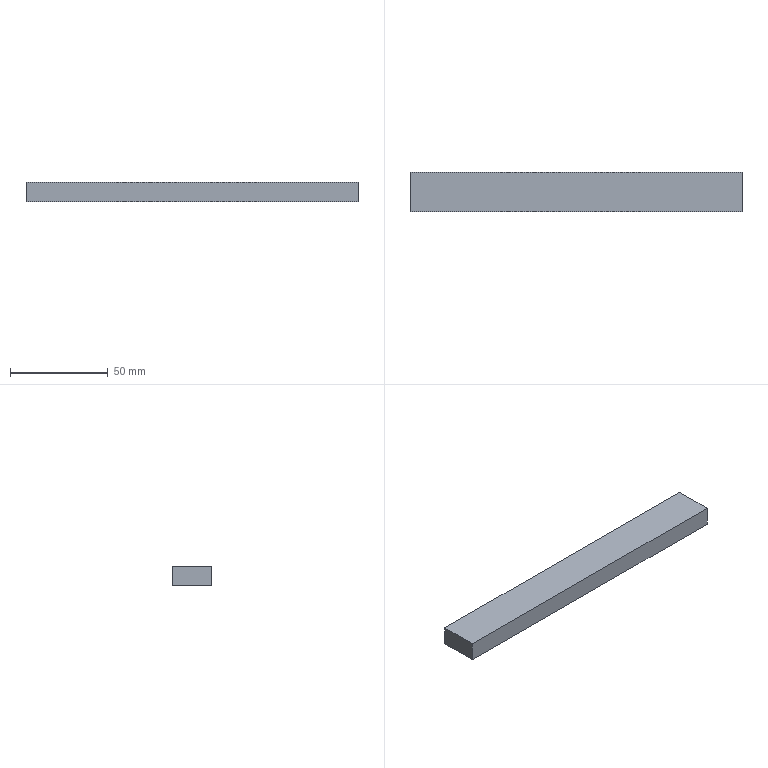Part | NX | features solid 2 | 1 solid | 6 faces | box 170 x 20 x 10 mm | volume 34000 mm3 | plane 6
STEP:
#1=CARTESIAN_POINT('',(85.,547.,-73.));
#2=VERTEX_POINT('',#1);
#3=CARTESIAN_POINT('',(85.,547.,-83.));
#4=VERTEX_POINT('',#3);
#5=CARTESIAN_POINT('',(85.,547.,-78.));
#6=DIRECTION('',(0.,0.,-1.));
#7=VECTOR('',#6,1000.);
#8=LINE('',#5,#7);
#9=EDGE_CURVE('',#2,#4,#8,.T.);
#10=ORIENTED_EDGE('',*,*,#9,.T.);
#11=CARTESIAN_POINT('',(-85.,547.,-83.));
#12=VERTEX_POINT('',#11);
#13=CARTESIAN_POINT('',(0.,547.,-83.));
#14=DIRECTION('',(-1.,0.,0.));
#15=VECTOR('',#14,1000.);
#16=LINE('',#13,#15);
#17=EDGE_CURVE('',#12,#4,#16,.F.);
#18=ORIENTED_EDGE('',*,*,#17,.F.);
#19=CARTESIAN_POINT('',(-85.,547.,-73.));
#20=VERTEX_POINT('',#19);
#21=CARTESIAN_POINT('',(-85.,547.,-78.));
#22=DIRECTION('',(0.,0.,-1.));
#23=VECTOR('',#22,1000.);
#24=LINE('',#21,#23);
#25=EDGE_CURVE('',#20,#12,#24,.T.);
#26=ORIENTED_EDGE('',*,*,#25,.F.);
#27=CARTESIAN_POINT('',(0.,547.,-73.));
#28=DIRECTION('',(-1.,0.,0.));
#29=VECTOR('',#28,1000.);
#30=LINE('',#27,#29);
#31=EDGE_CURVE('',#20,#2,#30,.F.);
#32=ORIENTED_EDGE('',*,*,#31,.T.);
#33=EDGE_LOOP('',(#10,#18,#26,#32));
#34=FACE_BOUND('',#33,.T.);
#35=CARTESIAN_POINT('',(0.,547.,-78.));
#36=DIRECTION('',(0.,1.,0.));
#37=DIRECTION('',(1.,0.,0.));
#38=AXIS2_PLACEMENT_3D('',#35,#36,#37);
#39=PLANE('',#38);
#40=ADVANCED_FACE('',(#34),#39,.T.);
#41=CARTESIAN_POINT('',(-85.,527.,-73.));
#42=VERTEX_POINT('',#41);
#43=CARTESIAN_POINT('',(85.,527.,-73.));
#44=VERTEX_POINT('',#43);
#45=CARTESIAN_POINT('',(0.,527.,-73.));
#46=DIRECTION('',(-1.,0.,0.));
#47=VECTOR('',#46,1000.);
#48=LINE('',#45,#47);
#49=EDGE_CURVE('',#42,#44,#48,.F.);
#50=ORIENTED_EDGE('',*,*,#49,.F.);
#51=CARTESIAN_POINT('',(-85.,527.,-83.));
#52=VERTEX_POINT('',#51);
#53=CARTESIAN_POINT('',(-85.,527.,-78.));
#54=DIRECTION('',(0.,0.,1.));
#55=VECTOR('',#54,1000.);
#56=LINE('',#53,#55);
#57=EDGE_CURVE('',#42,#52,#56,.F.);
#58=ORIENTED_EDGE('',*,*,#57,.T.);
#59=CARTESIAN_POINT('',(85.,527.,-83.));
#60=VERTEX_POINT('',#59);
#61=CARTESIAN_POINT('',(0.,527.,-83.));
#62=DIRECTION('',(-1.,0.,0.));
#63=VECTOR('',#62,1000.);
#64=LINE('',#61,#63);
#65=EDGE_CURVE('',#52,#60,#64,.F.);
#66=ORIENTED_EDGE('',*,*,#65,.T.);
#67=CARTESIAN_POINT('',(85.,527.,-78.));
#68=DIRECTION('',(0.,0.,1.));
#69=VECTOR('',#68,1000.);
#70=LINE('',#67,#69);
#71=EDGE_CURVE('',#44,#60,#70,.F.);
#72=ORIENTED_EDGE('',*,*,#71,.F.);
#73=EDGE_LOOP('',(#50,#58,#66,#72));
#74=FACE_BOUND('',#73,.T.);
#75=CARTESIAN_POINT('',(0.,527.,-78.));
#76=DIRECTION('',(0.,1.,0.));
#77=DIRECTION('',(1.,0.,0.));
#78=AXIS2_PLACEMENT_3D('',#75,#76,#77);
#79=PLANE('',#78);
#80=ADVANCED_FACE('',(#74),#79,.F.);
#81=CARTESIAN_POINT('',(85.,547.,-73.));
#82=DIRECTION('',(0.,1.,0.));
#83=VECTOR('',#82,1000.);
#84=LINE('',#81,#83);
#85=EDGE_CURVE('',#2,#44,#84,.F.);
#86=ORIENTED_EDGE('',*,*,#85,.T.);
#87=ORIENTED_EDGE('',*,*,#71,.T.);
#88=CARTESIAN_POINT('',(85.,547.,-83.));
#89=DIRECTION('',(0.,1.,0.));
#90=VECTOR('',#89,1000.);
#91=LINE('',#88,#90);
#92=EDGE_CURVE('',#4,#60,#91,.F.);
#93=ORIENTED_EDGE('',*,*,#92,.F.);
#94=ORIENTED_EDGE('',*,*,#9,.F.);
#95=EDGE_LOOP('',(#86,#87,#93,#94));
#96=FACE_BOUND('',#95,.T.);
#97=CARTESIAN_POINT('',(85.,547.,-78.));
#98=DIRECTION('',(1.,0.,0.));
#99=DIRECTION('',(0.,-1.,0.));
#100=AXIS2_PLACEMENT_3D('',#97,#98,#99);
#101=PLANE('',#100);
#102=ADVANCED_FACE('',(#96),#101,.T.);
#103=ORIENTED_EDGE('',*,*,#65,.F.);
#104=CARTESIAN_POINT('',(-85.,547.,-83.));
#105=DIRECTION('',(0.,1.,0.));
#106=VECTOR('',#105,1000.);
#107=LINE('',#104,#106);
#108=EDGE_CURVE('',#12,#52,#107,.F.);
#109=ORIENTED_EDGE('',*,*,#108,.F.);
#110=ORIENTED_EDGE('',*,*,#17,.T.);
#111=ORIENTED_EDGE('',*,*,#92,.T.);
#112=EDGE_LOOP('',(#103,#109,#110,#111));
#113=FACE_BOUND('',#112,.T.);
#114=CARTESIAN_POINT('',(0.,547.,-83.));
#115=DIRECTION('',(0.,0.,-1.));
#116=DIRECTION('',(-1.,0.,0.));
#117=AXIS2_PLACEMENT_3D('',#114,#115,#116);
#118=PLANE('',#117);
#119=ADVANCED_FACE('',(#113),#118,.T.);
#120=ORIENTED_EDGE('',*,*,#49,.T.);
#121=ORIENTED_EDGE('',*,*,#85,.F.);
#122=ORIENTED_EDGE('',*,*,#31,.F.);
#123=CARTESIAN_POINT('',(-85.,547.,-73.));
#124=DIRECTION('',(0.,1.,0.));
#125=VECTOR('',#124,1000.);
#126=LINE('',#123,#125);
#127=EDGE_CURVE('',#20,#42,#126,.F.);
#128=ORIENTED_EDGE('',*,*,#127,.T.);
#129=EDGE_LOOP('',(#120,#121,#122,#128));
#130=FACE_BOUND('',#129,.T.);
#131=CARTESIAN_POINT('',(0.,547.,-73.));
#132=DIRECTION('',(0.,0.,-1.));
#133=DIRECTION('',(-1.,0.,0.));
#134=AXIS2_PLACEMENT_3D('',#131,#132,#133);
#135=PLANE('',#134);
#136=ADVANCED_FACE('',(#130),#135,.F.);
#137=ORIENTED_EDGE('',*,*,#127,.F.);
#138=ORIENTED_EDGE('',*,*,#25,.T.);
#139=ORIENTED_EDGE('',*,*,#108,.T.);
#140=ORIENTED_EDGE('',*,*,#57,.F.);
#141=EDGE_LOOP('',(#137,#138,#139,#140));
#142=FACE_BOUND('',#141,.T.);
#143=CARTESIAN_POINT('',(-85.,547.,-78.));
#144=DIRECTION('',(-1.,0.,0.));
#145=DIRECTION('',(0.,-1.,0.));
#146=AXIS2_PLACEMENT_3D('',#143,#144,#145);
#147=PLANE('',#146);
#148=ADVANCED_FACE('',(#142),#147,.T.);
#149=CLOSED_SHELL('',(#40,#80,#102,#119,#136,#148));
#150=MANIFOLD_SOLID_BREP('',#149);
#151=(LENGTH_UNIT()NAMED_UNIT(*)SI_UNIT(.MILLI.,.METRE.));
#152=UNCERTAINTY_MEASURE_WITH_UNIT(LENGTH_MEASURE(0.00001),#151,'','');
#153=(NAMED_UNIT(*)PLANE_ANGLE_UNIT()SI_UNIT($,.RADIAN.));
#154=(NAMED_UNIT(*)SI_UNIT($,.STERADIAN.)SOLID_ANGLE_UNIT());
#155=(GEOMETRIC_REPRESENTATION_CONTEXT(3)GLOBAL_UNCERTAINTY_ASSIGNED_CONTEXT((#152))GLOBAL_UNIT_ASSIGNED_CONTEXT((#151,#153,#154))REPRESENTATION_CONTEXT('',''));
#156=ADVANCED_BREP_SHAPE_REPRESENTATION('',(#150),#155);